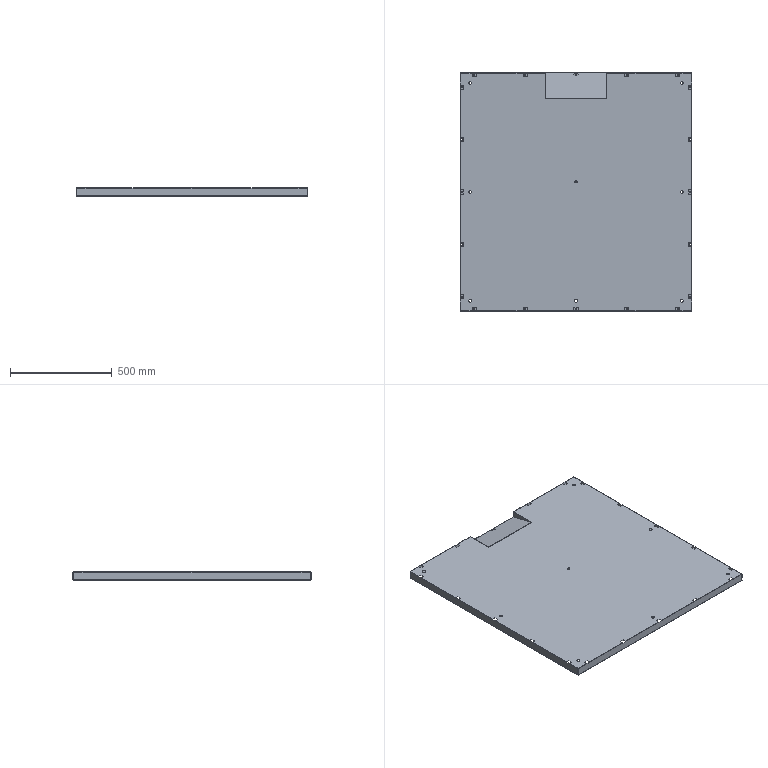Part | 2 solids | 400 faces | box 1139 x 1169 x 40 mm | volume 1567648 mm3 | plane 254 | cylinder 126 | spline 20 | commonest cylinder face diameters 7 x50 0.4 x30 2.4 x30 14 x14 11 x2